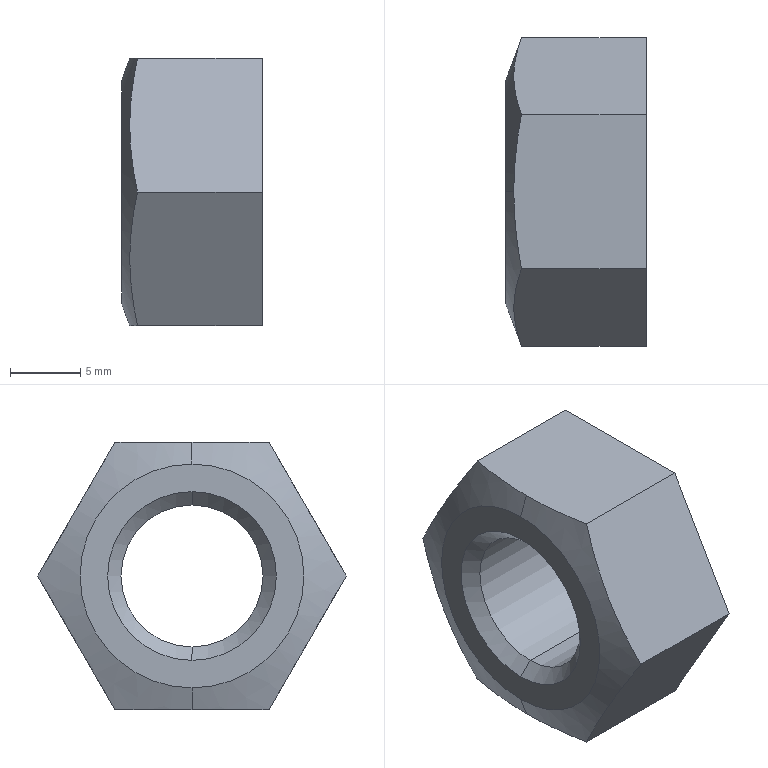Part | SolidWorks | features RefAxis 3, 3DProfileFeature 1, ICE 1, Revolution 1 | 1 solid | 16 faces | box 10 x 21.939 x 19 mm | volume 2247 mm3 | plane 8 | cone 6 | cylinder 2 | commonest cylinder face diameters 10.106 x2
STEP:
#1=CARTESIAN_POINT('',(9.053,0.,-5.053));
#2=VERTEX_POINT('',#1);
#3=CARTESIAN_POINT('',(9.053,0.,5.053));
#4=VERTEX_POINT('',#3);
#5=CARTESIAN_POINT('',(9.053,0.,0.));
#6=DIRECTION('',(-1.,0.,0.));
#7=DIRECTION('',(0.,0.,1.));
#8=AXIS2_PLACEMENT_3D('',#5,#6,#7);
#9=CIRCLE('',#8,5.053);
#10=EDGE_CURVE('',#2,#4,#9,.T.);
#11=ORIENTED_EDGE('',*,*,#10,.T.);
#12=CARTESIAN_POINT('',(10.,0.,6.));
#13=VERTEX_POINT('',#12);
#14=CARTESIAN_POINT('',(9.053,0.,5.053));
#15=DIRECTION('',(0.7071,0.,0.7071));
#16=VECTOR('',#15,1000.);
#17=LINE('',#14,#16);
#18=EDGE_CURVE('',#4,#13,#17,.T.);
#19=ORIENTED_EDGE('',*,*,#18,.T.);
#20=CARTESIAN_POINT('',(10.,0.,-6.));
#21=VERTEX_POINT('',#20);
#22=CARTESIAN_POINT('',(10.,0.,0.));
#23=DIRECTION('',(-1.,0.,0.));
#24=DIRECTION('',(0.,0.,1.));
#25=AXIS2_PLACEMENT_3D('',#22,#23,#24);
#26=CIRCLE('',#25,6.);
#27=EDGE_CURVE('',#21,#13,#26,.T.);
#28=ORIENTED_EDGE('',*,*,#27,.F.);
#29=CARTESIAN_POINT('',(9.053,0.,-5.053));
#30=DIRECTION('',(0.7071,0.,-0.7071));
#31=VECTOR('',#30,1000.);
#32=LINE('',#29,#31);
#33=EDGE_CURVE('',#2,#21,#32,.T.);
#34=ORIENTED_EDGE('',*,*,#33,.F.);
#35=EDGE_LOOP('',(#11,#19,#28,#34));
#36=FACE_OUTER_BOUND('',#35,.T.);
#37=CARTESIAN_POINT('',(9.053,0.,0.));
#38=DIRECTION('',(1.,0.,0.));
#39=DIRECTION('',(0.,0.,-1.));
#40=AXIS2_PLACEMENT_3D('',#37,#38,#39);
#41=CONICAL_SURFACE('',#40,5.053,0.7854);
#42=ADVANCED_FACE('',(#36),#41,.F.);
#43=ORIENTED_EDGE('',*,*,#10,.F.);
#44=CARTESIAN_POINT('',(0.947,0.,-5.053));
#45=VERTEX_POINT('',#44);
#46=CARTESIAN_POINT('',(10.,0.,-5.053));
#47=DIRECTION('',(-1.,0.,0.));
#48=VECTOR('',#47,1000.);
#49=LINE('',#46,#48);
#50=EDGE_CURVE('',#2,#45,#49,.T.);
#51=ORIENTED_EDGE('',*,*,#50,.T.);
#52=CARTESIAN_POINT('',(0.947,0.,5.053));
#53=VERTEX_POINT('',#52);
#54=CARTESIAN_POINT('',(0.947,0.,0.));
#55=DIRECTION('',(-1.,0.,0.));
#56=DIRECTION('',(0.,0.,1.));
#57=AXIS2_PLACEMENT_3D('',#54,#55,#56);
#58=CIRCLE('',#57,5.053);
#59=EDGE_CURVE('',#45,#53,#58,.T.);
#60=ORIENTED_EDGE('',*,*,#59,.T.);
#61=CARTESIAN_POINT('',(10.,0.,5.053));
#62=DIRECTION('',(-1.,0.,0.));
#63=VECTOR('',#62,1000.);
#64=LINE('',#61,#63);
#65=EDGE_CURVE('',#4,#53,#64,.T.);
#66=ORIENTED_EDGE('',*,*,#65,.F.);
#67=EDGE_LOOP('',(#43,#51,#60,#66));
#68=FACE_OUTER_BOUND('',#67,.T.);
#69=CARTESIAN_POINT('',(10.,0.,0.));
#70=DIRECTION('',(-1.,0.,0.));
#71=DIRECTION('',(0.,0.,1.));
#72=AXIS2_PLACEMENT_3D('',#69,#70,#71);
#73=CYLINDRICAL_SURFACE('',#72,5.053);
#74=ADVANCED_FACE('',(#68),#73,.F.);
#75=ORIENTED_EDGE('',*,*,#59,.F.);
#76=CARTESIAN_POINT('',(0.,0.,-6.));
#77=VERTEX_POINT('',#76);
#78=CARTESIAN_POINT('',(0.,0.,-6.));
#79=DIRECTION('',(-0.7071,0.,-0.7071));
#80=VECTOR('',#79,1000.);
#81=LINE('',#78,#80);
#82=EDGE_CURVE('',#45,#77,#81,.T.);
#83=ORIENTED_EDGE('',*,*,#82,.T.);
#84=CARTESIAN_POINT('',(0.,0.,6.));
#85=VERTEX_POINT('',#84);
#86=CARTESIAN_POINT('',(0.,0.,0.));
#87=DIRECTION('',(-1.,0.,0.));
#88=DIRECTION('',(0.,0.,1.));
#89=AXIS2_PLACEMENT_3D('',#86,#87,#88);
#90=CIRCLE('',#89,6.);
#91=EDGE_CURVE('',#77,#85,#90,.T.);
#92=ORIENTED_EDGE('',*,*,#91,.T.);
#93=CARTESIAN_POINT('',(0.,0.,6.));
#94=DIRECTION('',(-0.7071,0.,0.7071));
#95=VECTOR('',#94,1000.);
#96=LINE('',#93,#95);
#97=EDGE_CURVE('',#53,#85,#96,.T.);
#98=ORIENTED_EDGE('',*,*,#97,.F.);
#99=EDGE_LOOP('',(#75,#83,#92,#98));
#100=FACE_OUTER_BOUND('',#99,.T.);
#101=CARTESIAN_POINT('',(0.,0.,0.));
#102=DIRECTION('',(-1.,0.,0.));
#103=DIRECTION('',(0.,0.,1.));
#104=AXIS2_PLACEMENT_3D('',#101,#102,#103);
#105=CONICAL_SURFACE('',#104,6.,0.7854);
#106=ADVANCED_FACE('',(#100),#105,.F.);
#107=CARTESIAN_POINT('',(0.,0.,7.958));
#108=VERTEX_POINT('',#107);
#109=CARTESIAN_POINT('',(0.,0.,-7.958));
#110=VERTEX_POINT('',#109);
#111=CARTESIAN_POINT('',(0.,0.,0.));
#112=DIRECTION('',(-1.,0.,0.));
#113=DIRECTION('',(0.,0.,1.));
#114=AXIS2_PLACEMENT_3D('',#111,#112,#113);
#115=CIRCLE('',#114,7.958);
#116=EDGE_CURVE('',#108,#110,#115,.T.);
#117=ORIENTED_EDGE('',*,*,#116,.F.);
#118=CARTESIAN_POINT('',(0.5753,0.,9.5));
#119=VERTEX_POINT('',#118);
#120=CARTESIAN_POINT('',(1.462,0.,11.875));
#121=DIRECTION('',(0.3496,0.,0.9369));
#122=VECTOR('',#121,1000.);
#123=LINE('',#120,#122);
#124=EDGE_CURVE('',#108,#119,#123,.T.);
#125=ORIENTED_EDGE('',*,*,#124,.T.);
#126=CARTESIAN_POINT('',(1.124,5.485,9.5));
#127=VERTEX_POINT('',#126);
#128=CARTESIAN_POINT('',(0.5753,0.,9.5));
#129=CARTESIAN_POINT('',(0.5753,0.9159,9.5));
#130=CARTESIAN_POINT('',(0.6256,1.831,9.5));
#131=CARTESIAN_POINT('',(0.815,3.659,9.5));
#132=CARTESIAN_POINT('',(0.9538,4.574,9.5));
#133=CARTESIAN_POINT('',(1.124,5.485,9.5));
#134=B_SPLINE_CURVE_WITH_KNOTS('',3,(#128,#129,#130,#131,#132,#133),.UNSPECIFIED.,.F.,.F.,(4,2,4),(0.01485,0.01762,0.02039),.UNSPECIFIED.);
#135=EDGE_CURVE('',#119,#127,#134,.T.);
#136=ORIENTED_EDGE('',*,*,#135,.T.);
#137=CARTESIAN_POINT('',(1.124,10.97,0.));
#138=VERTEX_POINT('',#137);
#139=CARTESIAN_POINT('',(1.124,5.485,9.5));
#140=CARTESIAN_POINT('',(0.9531,5.942,8.708));
#141=CARTESIAN_POINT('',(0.8146,6.399,7.917));
#142=CARTESIAN_POINT('',(0.6254,7.313,6.333));
#143=CARTESIAN_POINT('',(0.5251,8.227,4.75));
#144=CARTESIAN_POINT('',(0.6254,9.141,3.167));
#145=CARTESIAN_POINT('',(0.8146,10.056,1.583));
#146=CARTESIAN_POINT('',(0.9531,10.513,0.7917));
#147=CARTESIAN_POINT('',(1.124,10.97,0.));
#148=B_SPLINE_CURVE_WITH_KNOTS('',3,(#139,#140,#141,#142,#143,#144,#145,#146,#147),.UNSPECIFIED.,.F.,.F.,(4,2,1,2,4),(0.000000231,0.002743,0.005485,0.008227,0.01097),.UNSPECIFIED.);
#149=EDGE_CURVE('',#127,#138,#148,.T.);
#150=ORIENTED_EDGE('',*,*,#149,.T.);
#151=CARTESIAN_POINT('',(1.124,5.485,-9.5));
#152=VERTEX_POINT('',#151);
#153=CARTESIAN_POINT('',(1.124,10.97,0.));
#154=CARTESIAN_POINT('',(0.9531,10.513,-0.7917));
#155=CARTESIAN_POINT('',(0.8146,10.056,-1.583));
#156=CARTESIAN_POINT('',(0.6254,9.141,-3.167));
#157=CARTESIAN_POINT('',(0.5251,8.227,-4.75));
#158=CARTESIAN_POINT('',(0.6254,7.313,-6.333));
#159=CARTESIAN_POINT('',(0.8146,6.399,-7.917));
#160=CARTESIAN_POINT('',(0.9531,5.942,-8.708));
#161=CARTESIAN_POINT('',(1.124,5.485,-9.5));
#162=B_SPLINE_CURVE_WITH_KNOTS('',3,(#153,#154,#155,#156,#157,#158,#159,#160,#161),.UNSPECIFIED.,.F.,.F.,(4,2,1,2,4),(0.000000231,0.002743,0.005485,0.008227,0.01097),.UNSPECIFIED.);
#163=EDGE_CURVE('',#138,#152,#162,.T.);
#164=ORIENTED_EDGE('',*,*,#163,.T.);
#165=CARTESIAN_POINT('',(0.5753,0.,-9.5));
#166=VERTEX_POINT('',#165);
#167=CARTESIAN_POINT('',(1.124,5.485,-9.5));
#168=CARTESIAN_POINT('',(0.9538,4.574,-9.5));
#169=CARTESIAN_POINT('',(0.815,3.659,-9.5));
#170=CARTESIAN_POINT('',(0.6256,1.831,-9.5));
#171=CARTESIAN_POINT('',(0.5753,0.9159,-9.5));
#172=CARTESIAN_POINT('',(0.5753,0.,-9.5));
#173=B_SPLINE_CURVE_WITH_KNOTS('',3,(#167,#168,#169,#170,#171,#172),.UNSPECIFIED.,.F.,.F.,(4,2,4),(0.01999,0.02276,0.02552),.UNSPECIFIED.);
#174=EDGE_CURVE('',#152,#166,#173,.T.);
#175=ORIENTED_EDGE('',*,*,#174,.T.);
#176=CARTESIAN_POINT('',(1.462,0.,-11.875));
#177=DIRECTION('',(0.3496,0.,-0.9369));
#178=VECTOR('',#177,1000.);
#179=LINE('',#176,#178);
#180=EDGE_CURVE('',#110,#166,#179,.T.);
#181=ORIENTED_EDGE('',*,*,#180,.F.);
#182=EDGE_LOOP('',(#117,#125,#136,#150,#164,#175,#181));
#183=FACE_OUTER_BOUND('',#182,.T.);
#184=CARTESIAN_POINT('',(1.462,0.,0.));
#185=DIRECTION('',(1.,0.,0.));
#186=DIRECTION('',(0.,0.,-1.));
#187=AXIS2_PLACEMENT_3D('',#184,#185,#186);
#188=CONICAL_SURFACE('',#187,11.875,1.214);
#189=ADVANCED_FACE('',(#183),#188,.T.);
#190=ORIENTED_EDGE('',*,*,#124,.F.);
#191=CARTESIAN_POINT('',(0.,0.,0.));
#192=DIRECTION('',(-1.,0.,0.));
#193=DIRECTION('',(0.,0.,1.));
#194=AXIS2_PLACEMENT_3D('',#191,#192,#193);
#195=CIRCLE('',#194,7.958);
#196=EDGE_CURVE('',#110,#108,#195,.T.);
#197=ORIENTED_EDGE('',*,*,#196,.F.);
#198=ORIENTED_EDGE('',*,*,#180,.T.);
#199=CARTESIAN_POINT('',(1.124,-5.485,-9.5));
#200=VERTEX_POINT('',#199);
#201=CARTESIAN_POINT('',(0.5753,0.,-9.5));
#202=CARTESIAN_POINT('',(0.5753,-0.9137,-9.5));
#203=CARTESIAN_POINT('',(0.6254,-1.828,-9.5));
#204=CARTESIAN_POINT('',(0.815,-3.659,-9.5));
#205=CARTESIAN_POINT('',(0.9544,-4.577,-9.5));
#206=CARTESIAN_POINT('',(1.124,-5.485,-9.5));
#207=B_SPLINE_CURVE_WITH_KNOTS('',3,(#201,#202,#203,#204,#205,#206),.UNSPECIFIED.,.F.,.F.,(4,2,4),(0.02552,0.02828,0.03103),.UNSPECIFIED.);
#208=EDGE_CURVE('',#166,#200,#207,.T.);
#209=ORIENTED_EDGE('',*,*,#208,.T.);
#210=CARTESIAN_POINT('',(1.124,-10.97,0.));
#211=VERTEX_POINT('',#210);
#212=CARTESIAN_POINT('',(1.124,-5.485,-9.5));
#213=CARTESIAN_POINT('',(0.9531,-5.942,-8.708));
#214=CARTESIAN_POINT('',(0.8146,-6.399,-7.917));
#215=CARTESIAN_POINT('',(0.6254,-7.313,-6.333));
#216=CARTESIAN_POINT('',(0.5251,-8.227,-4.75));
#217=CARTESIAN_POINT('',(0.6254,-9.141,-3.167));
#218=CARTESIAN_POINT('',(0.8146,-10.056,-1.583));
#219=CARTESIAN_POINT('',(0.9531,-10.513,-0.7917));
#220=CARTESIAN_POINT('',(1.124,-10.97,0.));
#221=B_SPLINE_CURVE_WITH_KNOTS('',3,(#212,#213,#214,#215,#216,#217,#218,#219,#220),.UNSPECIFIED.,.F.,.F.,(4,2,1,2,4),(0.000000231,0.002743,0.005485,0.008227,0.01097),.UNSPECIFIED.);
#222=EDGE_CURVE('',#200,#211,#221,.T.);
#223=ORIENTED_EDGE('',*,*,#222,.T.);
#224=CARTESIAN_POINT('',(1.124,-5.485,9.5));
#225=VERTEX_POINT('',#224);
#226=CARTESIAN_POINT('',(1.124,-10.97,0.));
#227=CARTESIAN_POINT('',(0.9531,-10.513,0.7917));
#228=CARTESIAN_POINT('',(0.8146,-10.056,1.583));
#229=CARTESIAN_POINT('',(0.6254,-9.141,3.167));
#230=CARTESIAN_POINT('',(0.5251,-8.227,4.75));
#231=CARTESIAN_POINT('',(0.6254,-7.313,6.333));
#232=CARTESIAN_POINT('',(0.8146,-6.399,7.917));
#233=CARTESIAN_POINT('',(0.9531,-5.942,8.708));
#234=CARTESIAN_POINT('',(1.124,-5.485,9.5));
#235=B_SPLINE_CURVE_WITH_KNOTS('',3,(#226,#227,#228,#229,#230,#231,#232,#233,#234),.UNSPECIFIED.,.F.,.F.,(4,2,1,2,4),(0.000000231,0.002743,0.005485,0.008227,0.01097),.UNSPECIFIED.);
#236=EDGE_CURVE('',#211,#225,#235,.T.);
#237=ORIENTED_EDGE('',*,*,#236,.T.);
#238=CARTESIAN_POINT('',(1.124,-5.485,9.5));
#239=CARTESIAN_POINT('',(0.9544,-4.577,9.5));
#240=CARTESIAN_POINT('',(0.815,-3.659,9.5));
#241=CARTESIAN_POINT('',(0.6254,-1.828,9.5));
#242=CARTESIAN_POINT('',(0.5753,-0.9137,9.5));
#243=CARTESIAN_POINT('',(0.5753,0.,9.5));
#244=B_SPLINE_CURVE_WITH_KNOTS('',3,(#238,#239,#240,#241,#242,#243),.UNSPECIFIED.,.F.,.F.,(4,2,4),(0.009323,0.01209,0.01485),.UNSPECIFIED.);
#245=EDGE_CURVE('',#225,#119,#244,.T.);
#246=ORIENTED_EDGE('',*,*,#245,.T.);
#247=EDGE_LOOP('',(#190,#197,#198,#209,#223,#237,#246));
#248=FACE_OUTER_BOUND('',#247,.T.);
#249=CARTESIAN_POINT('',(1.462,0.,0.));
#250=DIRECTION('',(1.,0.,0.));
#251=DIRECTION('',(0.,0.,-1.));
#252=AXIS2_PLACEMENT_3D('',#249,#250,#251);
#253=CONICAL_SURFACE('',#252,11.875,1.214);
#254=ADVANCED_FACE('',(#248),#253,.T.);
#255=CARTESIAN_POINT('',(0.,0.,0.));
#256=DIRECTION('',(-1.,0.,0.));
#257=DIRECTION('',(0.,0.,1.));
#258=AXIS2_PLACEMENT_3D('',#255,#256,#257);
#259=CIRCLE('',#258,6.);
#260=EDGE_CURVE('',#85,#77,#259,.T.);
#261=ORIENTED_EDGE('',*,*,#260,.F.);
#262=ORIENTED_EDGE('',*,*,#91,.F.);
#263=EDGE_LOOP('',(#261,#262));
#264=FACE_BOUND('',#263,.T.);
#265=ORIENTED_EDGE('',*,*,#196,.T.);
#266=ORIENTED_EDGE('',*,*,#116,.T.);
#267=EDGE_LOOP('',(#265,#266));
#268=FACE_OUTER_BOUND('',#267,.T.);
#269=CARTESIAN_POINT('',(0.,7.958,0.));
#270=DIRECTION('',(1.,0.,0.));
#271=DIRECTION('',(0.,0.,-1.));
#272=AXIS2_PLACEMENT_3D('',#269,#270,#271);
#273=PLANE('',#272);
#274=ADVANCED_FACE('',(#264,#268),#273,.F.);
#275=ORIENTED_EDGE('',*,*,#82,.F.);
#276=CARTESIAN_POINT('',(0.947,0.,0.));
#277=DIRECTION('',(-1.,0.,0.));
#278=DIRECTION('',(0.,0.,1.));
#279=AXIS2_PLACEMENT_3D('',#276,#277,#278);
#280=CIRCLE('',#279,5.053);
#281=EDGE_CURVE('',#53,#45,#280,.T.);
#282=ORIENTED_EDGE('',*,*,#281,.F.);
#283=ORIENTED_EDGE('',*,*,#97,.T.);
#284=ORIENTED_EDGE('',*,*,#260,.T.);
#285=EDGE_LOOP('',(#275,#282,#283,#284));
#286=FACE_OUTER_BOUND('',#285,.T.);
#287=CARTESIAN_POINT('',(0.,0.,0.));
#288=DIRECTION('',(-1.,0.,0.));
#289=DIRECTION('',(0.,0.,1.));
#290=AXIS2_PLACEMENT_3D('',#287,#288,#289);
#291=CONICAL_SURFACE('',#290,6.,0.7854);
#292=ADVANCED_FACE('',(#286),#291,.F.);
#293=ORIENTED_EDGE('',*,*,#50,.F.);
#294=CARTESIAN_POINT('',(9.053,0.,0.));
#295=DIRECTION('',(-1.,0.,0.));
#296=DIRECTION('',(0.,0.,1.));
#297=AXIS2_PLACEMENT_3D('',#294,#295,#296);
#298=CIRCLE('',#297,5.053);
#299=EDGE_CURVE('',#4,#2,#298,.T.);
#300=ORIENTED_EDGE('',*,*,#299,.F.);
#301=ORIENTED_EDGE('',*,*,#65,.T.);
#302=ORIENTED_EDGE('',*,*,#281,.T.);
#303=EDGE_LOOP('',(#293,#300,#301,#302));
#304=FACE_OUTER_BOUND('',#303,.T.);
#305=CARTESIAN_POINT('',(10.,0.,0.));
#306=DIRECTION('',(-1.,0.,0.));
#307=DIRECTION('',(0.,0.,1.));
#308=AXIS2_PLACEMENT_3D('',#305,#306,#307);
#309=CYLINDRICAL_SURFACE('',#308,5.053);
#310=ADVANCED_FACE('',(#304),#309,.F.);
#311=ORIENTED_EDGE('',*,*,#18,.F.);
#312=ORIENTED_EDGE('',*,*,#299,.T.);
#313=ORIENTED_EDGE('',*,*,#33,.T.);
#314=CARTESIAN_POINT('',(10.,0.,0.));
#315=DIRECTION('',(-1.,0.,0.));
#316=DIRECTION('',(0.,0.,1.));
#317=AXIS2_PLACEMENT_3D('',#314,#315,#316);
#318=CIRCLE('',#317,6.);
#319=EDGE_CURVE('',#13,#21,#318,.T.);
#320=ORIENTED_EDGE('',*,*,#319,.F.);
#321=EDGE_LOOP('',(#311,#312,#313,#320));
#322=FACE_OUTER_BOUND('',#321,.T.);
#323=CARTESIAN_POINT('',(9.053,0.,0.));
#324=DIRECTION('',(1.,0.,0.));
#325=DIRECTION('',(0.,0.,-1.));
#326=AXIS2_PLACEMENT_3D('',#323,#324,#325);
#327=CONICAL_SURFACE('',#326,5.053,0.7854);
#328=ADVANCED_FACE('',(#322),#327,.F.);
#329=CARTESIAN_POINT('',(10.,5.485,-9.5));
#330=VERTEX_POINT('',#329);
#331=CARTESIAN_POINT('',(10.,10.97,0.));
#332=VERTEX_POINT('',#331);
#333=CARTESIAN_POINT('',(10.,5.485,-9.5));
#334=DIRECTION('',(0.,0.5,0.866));
#335=VECTOR('',#334,1000.);
#336=LINE('',#333,#335);
#337=EDGE_CURVE('',#330,#332,#336,.T.);
#338=ORIENTED_EDGE('',*,*,#337,.T.);
#339=CARTESIAN_POINT('',(10.,5.485,9.5));
#340=VERTEX_POINT('',#339);
#341=CARTESIAN_POINT('',(10.,10.97,0.));
#342=DIRECTION('',(0.,-0.5,0.866));
#343=VECTOR('',#342,1000.);
#344=LINE('',#341,#343);
#345=EDGE_CURVE('',#332,#340,#344,.T.);
#346=ORIENTED_EDGE('',*,*,#345,.T.);
#347=CARTESIAN_POINT('',(10.,-5.485,9.5));
#348=VERTEX_POINT('',#347);
#349=CARTESIAN_POINT('',(10.,5.485,9.5));
#350=DIRECTION('',(0.,-1.,0.));
#351=VECTOR('',#350,1000.);
#352=LINE('',#349,#351);
#353=EDGE_CURVE('',#340,#348,#352,.T.);
#354=ORIENTED_EDGE('',*,*,#353,.T.);
#355=CARTESIAN_POINT('',(10.,-10.97,0.));
#356=VERTEX_POINT('',#355);
#357=CARTESIAN_POINT('',(10.,-5.485,9.5));
#358=DIRECTION('',(0.,-0.5,-0.866));
#359=VECTOR('',#358,1000.);
#360=LINE('',#357,#359);
#361=EDGE_CURVE('',#348,#356,#360,.T.);
#362=ORIENTED_EDGE('',*,*,#361,.T.);
#363=CARTESIAN_POINT('',(10.,-5.485,-9.5));
#364=VERTEX_POINT('',#363);
#365=CARTESIAN_POINT('',(10.,-10.97,0.));
#366=DIRECTION('',(0.,0.5,-0.866));
#367=VECTOR('',#366,1000.);
#368=LINE('',#365,#367);
#369=EDGE_CURVE('',#356,#364,#368,.T.);
#370=ORIENTED_EDGE('',*,*,#369,.T.);
#371=CARTESIAN_POINT('',(10.,-5.485,-9.5));
#372=DIRECTION('',(0.,1.,0.));
#373=VECTOR('',#372,1000.);
#374=LINE('',#371,#373);
#375=EDGE_CURVE('',#364,#330,#374,.T.);
#376=ORIENTED_EDGE('',*,*,#375,.T.);
#377=EDGE_LOOP('',(#338,#346,#354,#362,#370,#376));
#378=FACE_OUTER_BOUND('',#377,.T.);
#379=ORIENTED_EDGE('',*,*,#27,.T.);
#380=ORIENTED_EDGE('',*,*,#319,.T.);
#381=EDGE_LOOP('',(#379,#380));
#382=FACE_BOUND('',#381,.T.);
#383=CARTESIAN_POINT('',(10.,6.,0.));
#384=DIRECTION('',(-1.,0.,0.));
#385=DIRECTION('',(0.,0.,1.));
#386=AXIS2_PLACEMENT_3D('',#383,#384,#385);
#387=PLANE('',#386);
#388=ADVANCED_FACE('',(#378,#382),#387,.F.);
#389=CARTESIAN_POINT('',(10.,5.485,9.5));
#390=DIRECTION('',(-1.,0.,0.));
#391=VECTOR('',#390,1000.);
#392=LINE('',#389,#391);
#393=EDGE_CURVE('',#340,#127,#392,.T.);
#394=ORIENTED_EDGE('',*,*,#393,.F.);
#395=ORIENTED_EDGE('',*,*,#345,.F.);
#396=CARTESIAN_POINT('',(10.,10.97,0.));
#397=DIRECTION('',(-1.,0.,0.));
#398=VECTOR('',#397,1000.);
#399=LINE('',#396,#398);
#400=EDGE_CURVE('',#332,#138,#399,.T.);
#401=ORIENTED_EDGE('',*,*,#400,.T.);
#402=ORIENTED_EDGE('',*,*,#149,.F.);
#403=EDGE_LOOP('',(#394,#395,#401,#402));
#404=FACE_OUTER_BOUND('',#403,.T.);
#405=CARTESIAN_POINT('',(10.,10.97,0.));
#406=DIRECTION('',(0.,-0.866,-0.5));
#407=DIRECTION('',(0.,0.5,-0.866));
#408=AXIS2_PLACEMENT_3D('',#405,#406,#407);
#409=PLANE('',#408);
#410=ADVANCED_FACE('',(#404),#409,.F.);
#411=CARTESIAN_POINT('',(10.,-5.485,9.5));
#412=DIRECTION('',(-1.,0.,0.));
#413=VECTOR('',#412,1000.);
#414=LINE('',#411,#413);
#415=EDGE_CURVE('',#348,#225,#414,.T.);
#416=ORIENTED_EDGE('',*,*,#415,.F.);
#417=ORIENTED_EDGE('',*,*,#353,.F.);
#418=ORIENTED_EDGE('',*,*,#393,.T.);
#419=ORIENTED_EDGE('',*,*,#135,.F.);
#420=ORIENTED_EDGE('',*,*,#245,.F.);
#421=EDGE_LOOP('',(#416,#417,#418,#419,#420));
#422=FACE_OUTER_BOUND('',#421,.T.);
#423=CARTESIAN_POINT('',(10.,5.485,9.5));
#424=DIRECTION('',(0.,0.,-1.));
#425=DIRECTION('',(-1.,0.,0.));
#426=AXIS2_PLACEMENT_3D('',#423,#424,#425);
#427=PLANE('',#426);
#428=ADVANCED_FACE('',(#422),#427,.F.);
#429=CARTESIAN_POINT('',(10.,-10.97,0.));
#430=DIRECTION('',(-1.,0.,0.));
#431=VECTOR('',#430,1000.);
#432=LINE('',#429,#431);
#433=EDGE_CURVE('',#356,#211,#432,.T.);
#434=ORIENTED_EDGE('',*,*,#433,.F.);
#435=ORIENTED_EDGE('',*,*,#361,.F.);
#436=ORIENTED_EDGE('',*,*,#415,.T.);
#437=ORIENTED_EDGE('',*,*,#236,.F.);
#438=EDGE_LOOP('',(#434,#435,#436,#437));
#439=FACE_OUTER_BOUND('',#438,.T.);
#440=CARTESIAN_POINT('',(10.,-5.485,9.5));
#441=DIRECTION('',(0.,0.866,-0.5));
#442=DIRECTION('',(0.,0.5,0.866));
#443=AXIS2_PLACEMENT_3D('',#440,#441,#442);
#444=PLANE('',#443);
#445=ADVANCED_FACE('',(#439),#444,.F.);
#446=CARTESIAN_POINT('',(10.,-5.485,-9.5));
#447=DIRECTION('',(-1.,0.,0.));
#448=VECTOR('',#447,1000.);
#449=LINE('',#446,#448);
#450=EDGE_CURVE('',#364,#200,#449,.T.);
#451=ORIENTED_EDGE('',*,*,#450,.F.);
#452=ORIENTED_EDGE('',*,*,#369,.F.);
#453=ORIENTED_EDGE('',*,*,#433,.T.);
#454=ORIENTED_EDGE('',*,*,#222,.F.);
#455=EDGE_LOOP('',(#451,#452,#453,#454));
#456=FACE_OUTER_BOUND('',#455,.T.);
#457=CARTESIAN_POINT('',(10.,-10.97,0.));
#458=DIRECTION('',(0.,0.866,0.5));
#459=DIRECTION('',(0.,-0.5,0.866));
#460=AXIS2_PLACEMENT_3D('',#457,#458,#459);
#461=PLANE('',#460);
#462=ADVANCED_FACE('',(#456),#461,.F.);
#463=CARTESIAN_POINT('',(10.,5.485,-9.5));
#464=DIRECTION('',(-1.,0.,0.));
#465=VECTOR('',#464,1000.);
#466=LINE('',#463,#465);
#467=EDGE_CURVE('',#330,#152,#466,.T.);
#468=ORIENTED_EDGE('',*,*,#467,.F.);
#469=ORIENTED_EDGE('',*,*,#375,.F.);
#470=ORIENTED_EDGE('',*,*,#450,.T.);
#471=ORIENTED_EDGE('',*,*,#208,.F.);
#472=ORIENTED_EDGE('',*,*,#174,.F.);
#473=EDGE_LOOP('',(#468,#469,#470,#471,#472));
#474=FACE_OUTER_BOUND('',#473,.T.);
#475=CARTESIAN_POINT('',(10.,-5.485,-9.5));
#476=DIRECTION('',(0.,0.,1.));
#477=DIRECTION('',(1.,0.,0.));
#478=AXIS2_PLACEMENT_3D('',#475,#476,#477);
#479=PLANE('',#478);
#480=ADVANCED_FACE('',(#474),#479,.F.);
#481=ORIENTED_EDGE('',*,*,#400,.F.);
#482=ORIENTED_EDGE('',*,*,#337,.F.);
#483=ORIENTED_EDGE('',*,*,#467,.T.);
#484=ORIENTED_EDGE('',*,*,#163,.F.);
#485=EDGE_LOOP('',(#481,#482,#483,#484));
#486=FACE_OUTER_BOUND('',#485,.T.);
#487=CARTESIAN_POINT('',(10.,5.485,-9.5));
#488=DIRECTION('',(0.,-0.866,0.5));
#489=DIRECTION('',(0.,-0.5,-0.866));
#490=AXIS2_PLACEMENT_3D('',#487,#488,#489);
#491=PLANE('',#490);
#492=ADVANCED_FACE('',(#486),#491,.F.);
#493=CLOSED_SHELL('',(#42,#74,#106,#189,#254,#274,#292,#310,#328,#388,#410,#428,#445,#462,#480,#492));
#494=MANIFOLD_SOLID_BREP('',#493);
#495=CARTESIAN_POINT('',(0.,0.,0.));
#496=DIRECTION('',(0.,0.,1.));
#497=DIRECTION('',(1.,0.,0.));
#498=AXIS2_PLACEMENT_3D('',#495,#496,#497);
#499=(LENGTH_UNIT()NAMED_UNIT(*)SI_UNIT(.MILLI.,.METRE.));
#500=UNCERTAINTY_MEASURE_WITH_UNIT(LENGTH_MEASURE(0.00001),#499,'','');
#501=(NAMED_UNIT(*)PLANE_ANGLE_UNIT()SI_UNIT($,.RADIAN.));
#502=(NAMED_UNIT(*)SI_UNIT($,.STERADIAN.)SOLID_ANGLE_UNIT());
#503=(GEOMETRIC_REPRESENTATION_CONTEXT(3)GLOBAL_UNCERTAINTY_ASSIGNED_CONTEXT((#500))GLOBAL_UNIT_ASSIGNED_CONTEXT((#499,#501,#502))REPRESENTATION_CONTEXT('',''));
#504=ADVANCED_BREP_SHAPE_REPRESENTATION('',(#494,#498),#503);